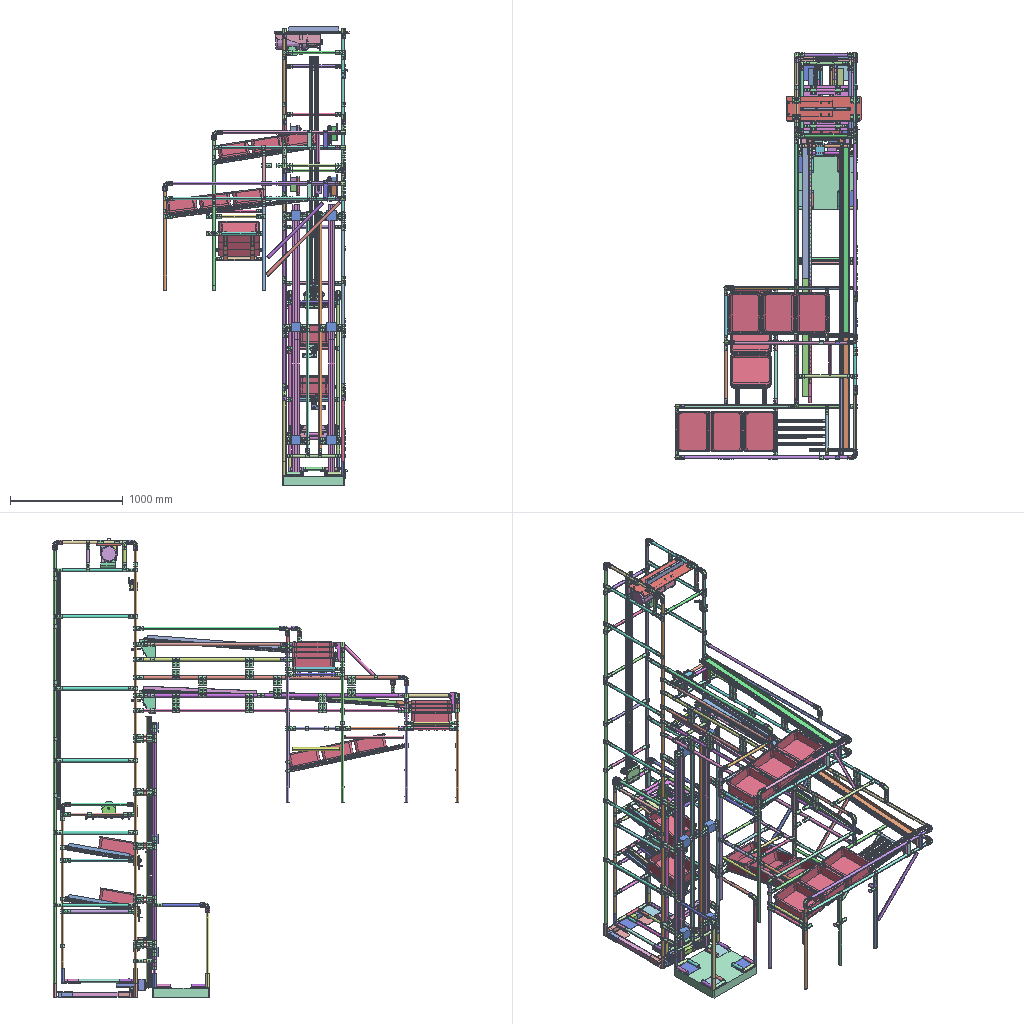Assembly | STEP file | 145 different items | 1167 placed | box 1651 x 3605 x 4075 mm
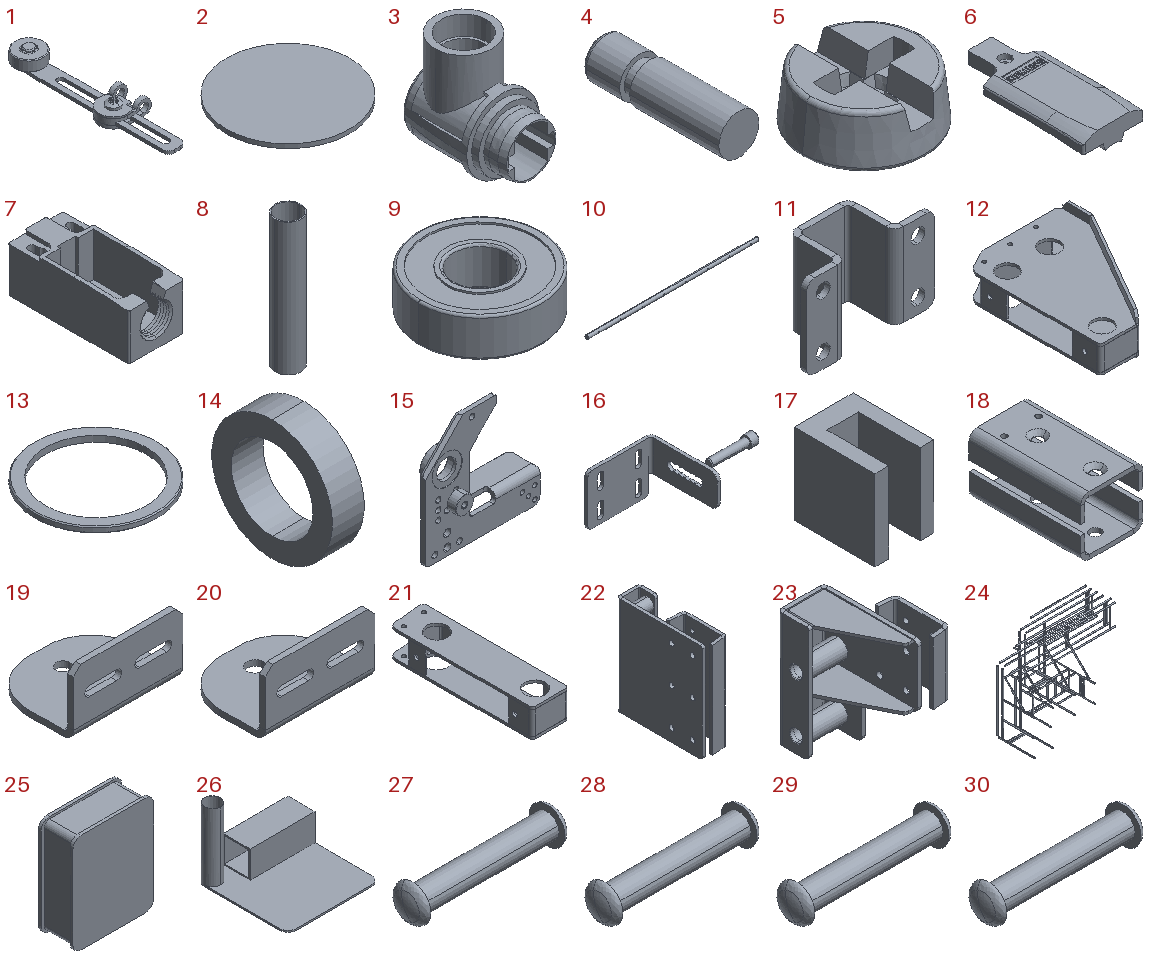Parts list (item | name | quantity | parent item | size | volume):
1 | 2023_07_21_12_39_19_0122 | x2 | in cc_unnamed | 25.5 x 109 x 14 mm | 5452 mm3
2 | 2023_07_21_12_39_19_0126 | x2 | in cc_unnamed | 18 x 18 x 0.6 mm | 152.681 mm3
3 | 2023_07_21_12_39_19_0129 | x2 | in cc_unnamed | 24.025 x 33.5 x 35.012 mm | 7738 mm3
4 | 2023_07_21_12_39_19_0133 | x2 | in cc_unnamed | 7 x 24.6 x 7 mm | 901.225 mm3
5 | 2023_07_21_12_39_19_0137 | x2 | in cc_unnamed | 5.956 x 5.956 x 2.4 mm | 49.622 mm3
6 | 2023_07_21_12_39_19_0141 | x2 | in cc_unnamed | 31 x 68 x 10.875 mm | 10432 mm3
7 | 2023_07_21_12_39_19_0144 | x2 | in cc_unnamed | 31 x 68 x 27 mm | 22352 mm3
8 | 28._28.6X145 | x32 | in SOPORTE DOBLE, Soporte riel_Completo | 28.6 x 28.6 x 145 mm | 14978 mm3
9 | 6202RS | x22 | in POLEA IZAJE ASSY, RODAJA ENSAMBLE, RODAJA ENSAMBLE SUPERIOR, RODAJA FRONTAL | 35 x 35 x 11 mm | 8156 mm3
10 | 6499K55_Shaft for Support Rail_6499K55 | x4 | in RIEL_ASSY | 1200 x 25 x 25 mm | 586134 mm3
11 | ABRAZADERA a | x8 | in ELEVADOR REV 09-03-26 ASSY, ENSAMBLE BASE IZAJE | 77 x 31.7 x 50 mm | 21367 mm3
12 | ACTIVACION MECANICA UPPER RH SLIM V2.1_SLIM V3<Como mecanizada> | x2 | in CAIDA AV3 | 145 x 200 x 60 mm | 208719 mm3
13 | ARANDELA INT. RODAJA | x8 | in RODAJA ENSAMBLE, RODAJA ENSAMBLE SUPERIOR | 18.5 x 18.5 x 0.9 mm | 78.382 mm3
14 | ARANDELA POSTERIOR BALANCIN | x1 | in MECANISMO BALANCIN | 4.76 x 18 x 18 mm | 654.835 mm3
15 | BALANCIN | x1 | in MECANISMO BALANCIN | 130 x 45 x 130 mm | 53768 mm3
16 | BASE ACTIVACION BALANCIN | x1 | in CAIDA AV3 | 205 x 110 x 80 mm | 64247 mm3
17 | BASE GUIA LINEAL_A | x6 | in Soporte riel_Completo | 62 x 85 x 85 mm | 265625 mm3
18 | BASE MICRO | x2 | in cc_unnamed | 38 x 68 x 36 mm | 20484 mm3
19 | BASE POLEA_B_SHEET METAL | x1 | in POLEA IZAJE ASSY | 120 x 100 x 70 mm | 108585 mm3
20 | BASE POLEA_SHEET METAL | x1 | in POLEA IZAJE ASSY | 120 x 100 x 70 mm | 108092 mm3
21 | BASE RIEL SUPERIOR_SLIM V2 | x1 | in CAIDA AV3 | 50 x 199.37 x 39 mm | 75917 mm3
22 | BASE RODILLOS FRONTALES | x1 | in BASE RODILLOS FRONTALES UP | 38.52 x 144.159 x 160 mm | 238623 mm3
23 | BASE RODILLOS SUPERIORES_BASE CONTRA PLACA | x1 | in CANASTA MODIFICACION MECANISMO RETRACTIL | 93.76 x 131.085 x 148 mm | 235886 mm3
24 | CAIDA A V3_Predeterminado<Como mecanizada> | x1 | in CAIDA AV3 | 2864 x 1554 x 1609 mm | 6177747 mm3
25 | CONTENEDOR TORNILLOS | x11 | in CAIDA AV3, CANASTA MODIFICACION MECANISMO RETRACTIL | 292 x 125 x 360 mm | 3821373 mm3
26 | Component1 | x4 | in MB-P | 170 x 170 x 128 mm | 151175 mm3
27 | Component10 | x1 | in Rieles_1 | 25.4 x 6 x 6 mm | 338.091 mm3
28 | Component11 | x1 | in Rieles_1 | 25.4 x 6 x 6 mm | 338.091 mm3
29 | Component12 | x1 | in Rieles_1 | 25.4 x 6 x 6 mm | 338.091 mm3
30 | Component13 | x1 | in Rieles_1 | 25.4 x 6 x 6 mm | 338.091 mm3
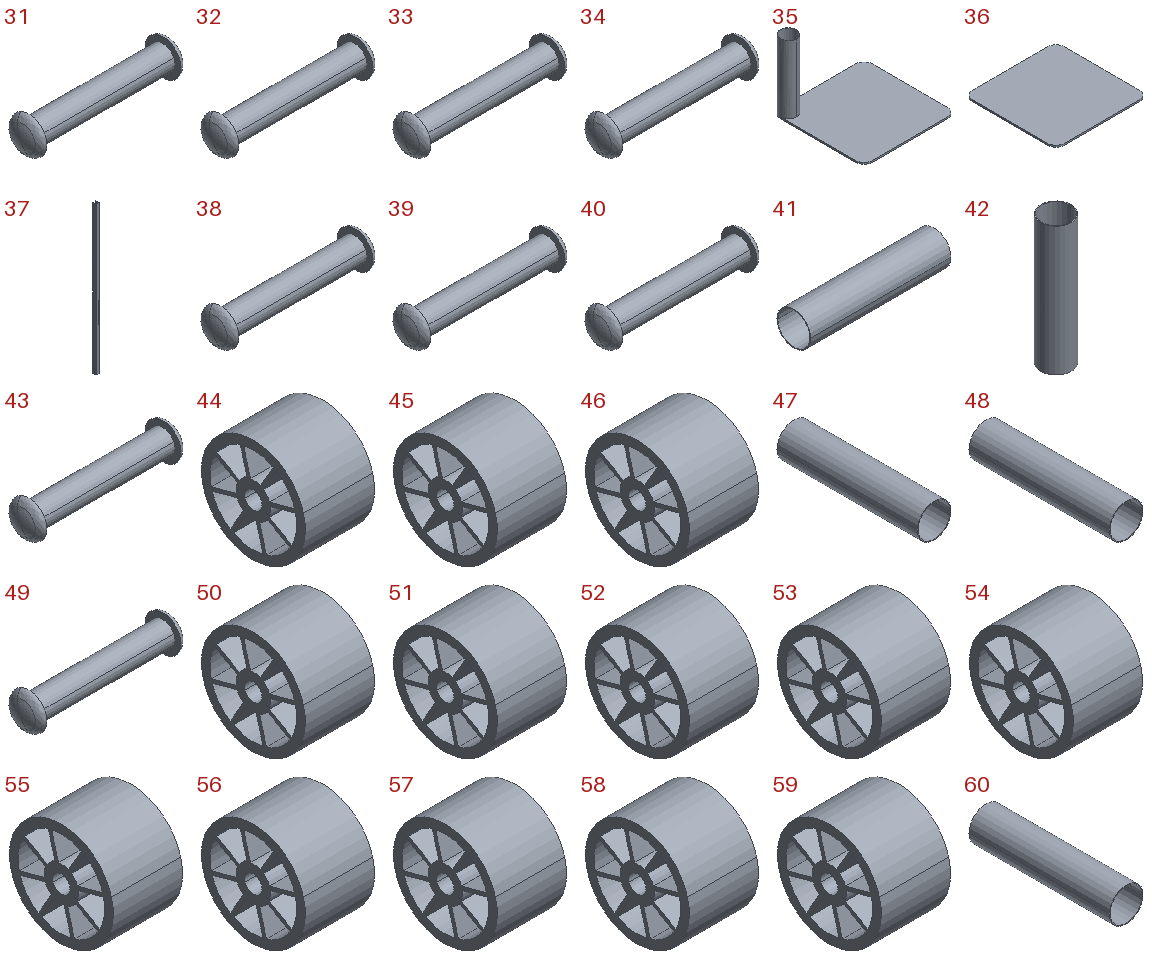31 | Component14 | x1 | in Rieles_1 | 25.4 x 6 x 6 mm | 338.059 mm3
32 | Component15 | x1 | in Rieles_1 | 25.4 x 6 x 6 mm | 338.067 mm3
33 | Component16 | x1 | in Rieles_1 | 25.4 x 6 x 6 mm | 338.067 mm3
34 | Component17 | x1 | in Rieles_1 | 25.4 x 6 x 6 mm | 338.091 mm3
35 | Component1_1 | x4 | in YT-R, YT-R_2 | 170 x 170 x 128 mm | 94175 mm3
36 | Component1_2 | x4 | in YT-L_1, YT-L_3 | 170 x 170 x 3 mm | 86121 mm3
37 | Component2 | x1 | in Rieles_1 | 28.4 x 26.2 x 1238 mm | 123368 mm3
38 | Component25 | x1 | in Rieles_1 | 25.4 x 6 x 6 mm | 338.067 mm3
39 | Component26 | x1 | in Rieles_1 | 25.4 x 6 x 6 mm | 338.067 mm3
40 | Component27 | x1 | in Rieles_1 | 25.4 x 6 x 6 mm | 338.091 mm3
41 | Component2_1 | x4 | in YT-R, YT-R_2 | 125 x 30 x 30 mm | 8054 mm3
42 | Component2_2 | x4 | in YT-L_1, YT-L_3 | 30 x 30 x 125 mm | 8054 mm3
43 | Component3 | x1 | in Rieles_1 | 25.4 x 6 x 6 mm | 338.067 mm3
44 | Component37 | x18 | in Rieles_1 | 20 x 30 x 30 mm | 6699 mm3
45 | Component38 | x1 | in Rieles_1 | 20 x 30 x 30 mm | 6699 mm3
46 | Component39 | x1 | in Rieles_1 | 20 x 30 x 30 mm | 6699 mm3
47 | Component3_1 | x4 | in YT-R, YT-R_2 | 30 x 125 x 30 mm | 8054 mm3
48 | Component3_2 | x4 | in YT-L_1, YT-L_3 | 30 x 125 x 30 mm | 8054 mm3
49 | Component4 | x1 | in Rieles_1 | 25.4 x 6 x 6 mm | 338.067 mm3
50 | Component40 | x1 | in Rieles_1 | 20 x 30 x 30 mm | 6699 mm3
51 | Component41 | x1 | in Rieles_1 | 20 x 30 x 30 mm | 6699 mm3
52 | Component42 | x1 | in Rieles_1 | 20 x 30 x 30 mm | 6699 mm3
53 | Component43 | x1 | in Rieles_1 | 20 x 30 x 30 mm | 6699 mm3
54 | Component44 | x1 | in Rieles_1 | 20 x 30 x 30 mm | 6699 mm3
55 | Component45 | x1 | in Rieles_1 | 20 x 30 x 30 mm | 6699 mm3
56 | Component46 | x1 | in Rieles_1 | 20 x 30 x 30 mm | 6699 mm3
57 | Component47 | x1 | in Rieles_1 | 20 x 30 x 30 mm | 6699 mm3
58 | Component48 | x1 | in Rieles_1 | 20 x 30 x 30 mm | 6699 mm3
59 | Component49 | x1 | in Rieles_1 | 20 x 30 x 30 mm | 6699 mm3
60 | Component4_1 | x4 | in YT-R, YT-R_2 | 30 x 125 x 30 mm | 8054 mm3
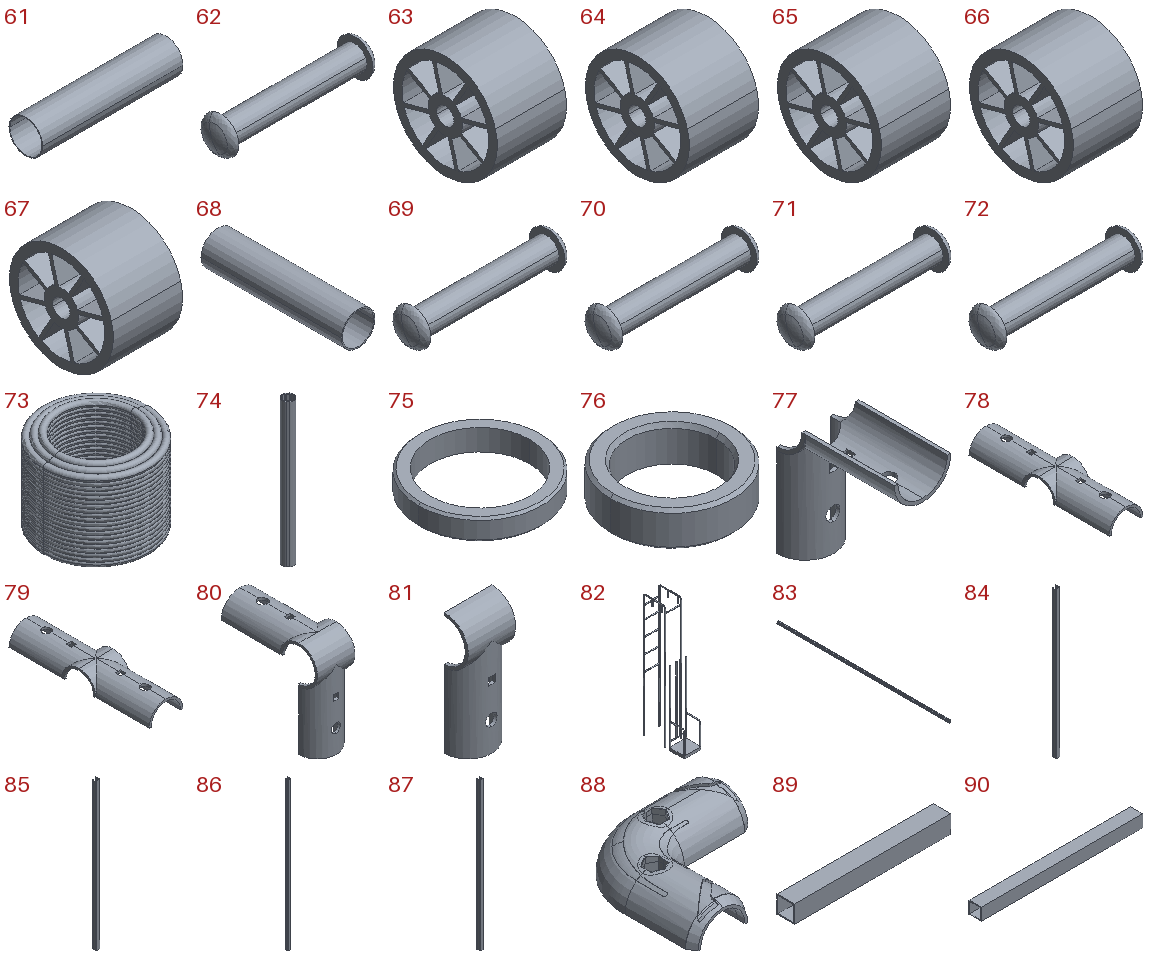61 | Component4_2 | x4 | in YT-L_1, YT-L_3 | 125 x 30 x 30 mm | 8054 mm3
62 | Component5 | x1 | in Rieles_1 | 25.4 x 6 x 6 mm | 338.091 mm3
63 | Component50 | x1 | in Rieles_1 | 20 x 30 x 30 mm | 6699 mm3
64 | Component51 | x1 | in Rieles_1 | 20 x 30 x 30 mm | 6699 mm3
65 | Component52 | x1 | in Rieles_1 | 20 x 30 x 30 mm | 6699 mm3
66 | Component53 | x1 | in Rieles_1 | 20 x 30 x 30 mm | 6699 mm3
67 | Component54 | x117 | in RIEL 1_02, RIEL 2_24, RIEL NIVEL 2-23, RIEL2_02, Rieles_1 | 20 x 30 x 30 mm | 6699 mm3
68 | Component5_1 | x4 | in YT-L_1, YT-L_3 | 30 x 125 x 30 mm | 11388 mm3
69 | Component6 | x1 | in Rieles_1 | 25.4 x 6 x 6 mm | 338.091 mm3
70 | Component7 | x1 | in Rieles_1 | 25.4 x 6 x 6 mm | 338.091 mm3
71 | Component8 | x1 | in Rieles_1 | 25.4 x 6 x 6 mm | 338.091 mm3
72 | Component9 | x1 | in Rieles_1 | 25.4 x 6 x 6 mm | 338.091 mm3
73 | Cable Rep^Pittsburgh Automotive 1300lb remote controlled electric hoist - Representation | x1 | in Pittsburgh Automotive 1300lb remote controlled electric hoist - Representation | 107.694 x 107.694 x 86.428 mm | 372136 mm3
74 | DROP STOP 1 ALUMINUM_Default<As machined> | x2 | in TOPE C1 ALUM | 30 x 30 x 380 mm | 75887 mm3
75 | ESPACIADOR POLEA | x1 | in POLEA IZAJE ASSY | 34.9 x 34.9 x 6 mm | 2006 mm3
76 | ESPACIADOR POLEA 2 | x1 | in POLEA IZAJE ASSY | 21 x 21 x 6 mm | 965.28 mm3
77 | F-A | x22 | in F-A_&_F-C_16, F-A_&_F-C_6 | 32.6 x 67.3 x 67.3 mm | 10224 mm3
78 | F-B | x5 | in F-B_F-B_2 | 32.6 x 134.6 x 16.3 mm | 12017 mm3
79 | F-B_F-B_2-2 | x5 | in F-B_F-B_2 | 32.6 x 134.6 x 16.3 mm | 12017 mm3
80 | F-C | x22 | in F-A_&_F-C_16, F-A_&_F-C_6 | 32.6 x 83.6 x 83.6 mm | 13591 mm3
81 | F-D | x574 | in F-D_F-D_24, F-D_F-D_26, F-D_F-D_27, F-D_F-D_9 | 32.6 x 16.3 x 83.6 mm | 7578 mm3
82 | FRAME ESTRUCTURA REV 3_Predeterminado<Como mecanizada> | x1 | in ELEVADOR REV 09-03-26 ASSY | 552 x 1382 x 4049 mm | 25982334 mm3
83 | FRONT GUIDE_ALUMINUM TUBE ITEM<As machined> | x2 | in GUIAS FRONTALES | 30 x 2110 x 30 mm | 421372 mm3
84 | GALVANIZED RAIL | x1 | in RIEL 1_02 | 28.4 x 26.2 x 999 mm | 99436 mm3
85 | GALVANIZED RAIL 02 | x1 | in RIEL2_02 | 28.4 x 26.2 x 999 mm | 99426 mm3
86 | GALVANIZED RAIL 023 | x1 | in RIEL NIVEL 2-23 | 28.4 x 26.2 x 1678 mm | 167389 mm3
87 | GALVANIZED RAIL 24 | x1 | in RIEL 2_24 | 28.4 x 26.2 x 1218 mm | 121365 mm3
88 | GT-90D | x44 | in HJ13, HJ13_3 | 89.055 x 89.077 x 19.235 mm | 46571 mm3
89 | MB-360X400 | x2 | in ELEVADOR REV 09-03-26 ASSY | 400 x 45 x 45 mm | 170000 mm3
90 | MB-360X600 | x2 | in ELEVADOR REV 09-03-26 ASSY | 600 x 45 x 45 mm | 255000 mm3
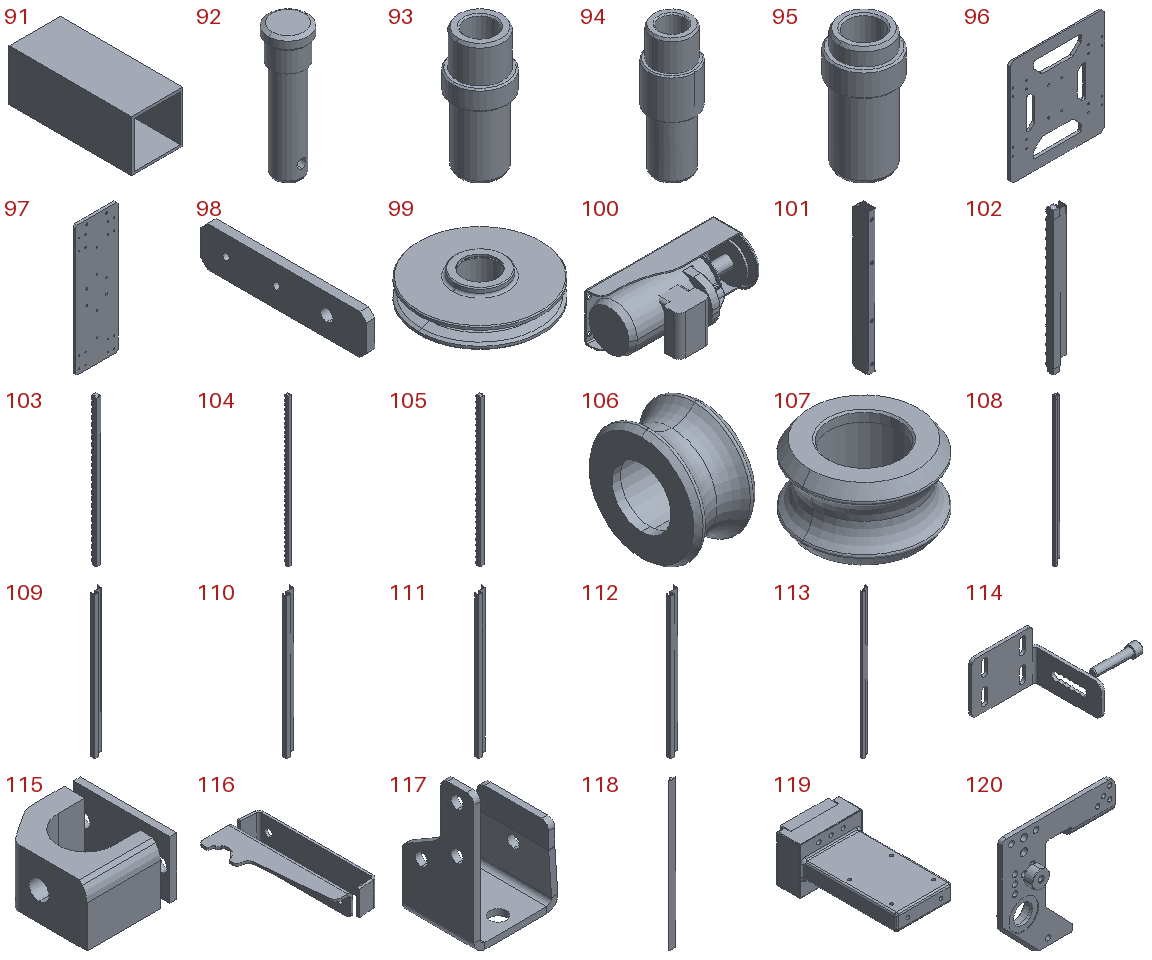91 | MB-P-20 | x4 | in MB-P | 50 x 120 x 50 mm | 57000 mm3
92 | PERNO POLEA_PERNO V2 | x1 | in POLEA IZAJE ASSY | 21 x 21 x 69 mm | 13594 mm3
93 | PERNO RODAJA FRONTAL | x2 | in BASE RODILLOS FRONTALES UP | 19 x 19 x 42.7 mm | 5059 mm3
94 | PERNO RODAJA SUPERIOR | x4 | in RODAJA ENSAMBLE SUPERIOR | 19 x 19 x 52.7 mm | 7077 mm3
95 | PLACA BASE EXCENTRICA | x4 | in RODAJA ENSAMBLE | 18 x 18 x 35.7 mm | 3926 mm3
96 | PLACA BASE IZAJE | x1 | in ENSAMBLE BASE IZAJE | 400 x 12 x 450 mm | 1745930 mm3
97 | PLACA BASE POLIPASTO | x1 | in 97 | 220 x 12 x 665 mm | 1721433 mm3
98 | PLACA SOPORTE GUIA | x2 | in GUIAS FRONTALES | 6.35 x 125 x 30 mm | 22842 mm3
99 | POLEA IZAJE_MAMELON | x1 | in POLEA IZAJE ASSY | 125 x 125 x 35 mm | 205749 mm3
100 | Pittsburgh Hoist^Pittsburgh Automotive 1300lb remote controlled electric hoist - Representation | x1 | in Pittsburgh Automotive 1300lb remote controlled electric hoist - Representation | 415.037 x 200.01 x 149.835 mm | 6132353 mm3
101 | REFUERZO PLACA BASE POLIPASTO | x1 | in 97 | 25.4 x 50.8 x 450 mm | 118043 mm3
102 | RIEL CABINA | x2 | in CANASTA MODIFICACION MECANISMO RETRACTIL | 81.4 x 57.7 x 600 mm | 321427 mm3
103 | RIEL FINAL NLV 1 | x4 | in CAIDA AV3 | 28.4 x 36.2 x 873.5 mm | 257286 mm3
104 | RIEL FINAL NLV 2 | x4 | in CAIDA AV3 | 28.4 x 36.2 x 1308 mm | 381210 mm3
105 | RIEL FINAL NLV 3 | x2 | in CAIDA AV3 | 28.4 x 36.2 x 1045 mm | 307295 mm3
106 | RODAJA D29 | x2 | in RODAJA FRONTAL | 32 x 59.25 x 59.25 mm | 39424 mm3
107 | ROLLER LINEAR GUIDE_01 | x8 | in RODAJA ENSAMBLE, RODAJA ENSAMBLE SUPERIOR | 55.257 x 55.257 x 32 mm | 32346 mm3
108 | Rieles | x1 | in CAIDA AV3 | 81.4 x 57.7 x 1724 mm | 936663 mm3
109 | Rieles_1-21 | x1 | in Rieles_1 | 81.4 x 57.7 x 1164 mm | 303280 mm3
110 | Rieles_1-22 | x1 | in RIEL 1_02 | 81.4 x 57.7 x 1003 mm | 261332 mm3
111 | Rieles_1-24 | x1 | in RIEL 2_24 | 81.4 x 57.7 x 1129 mm | 294161 mm3
112 | Rieles_2-22 | x1 | in RIEL2_02 | 81.4 x 57.7 x 999 mm | 260289 mm3
113 | Rieles_2-23 | x1 | in RIEL NIVEL 2-23 | 81.4 x 57.7 x 1608 mm | 418964 mm3
114 | SIMETRIA BASE ACTIVACION | x1 | in CAIDA AV3 | 205 x 110 x 80 mm | 64247 mm3
115 | SOPORTE BALANCIN | x1 | in MECANISMO BALANCIN | 46.5 x 50 x 30 mm | 35322 mm3
116 | SOPORTE ITEM | x2 | in TOPE C1 ALUM | 83.5 x 174.166 x 35 mm | 61549 mm3
117 | SOPORTE RESORTE 1 | x1 | in CANASTA MODIFICACION MECANISMO RETRACTIL | 35.055 x 30 x 57.6 mm | 7586 mm3
118 | SOPORTE RIEL 25mm | x4 | in RIEL_ASSY | 55 x 21.275 x 1200 mm | 648615 mm3
119 | Sopote_cabina | x2 | in CANASTA MODIFICACION MECANISMO RETRACTIL | 134.1 x 257 x 100 mm | 1531756 mm3
120 | Symmetry BALANCER 01 | x1 | in Symmetry BALANCER MECHANISM | 130 x 45 x 130 mm | 53768 mm3
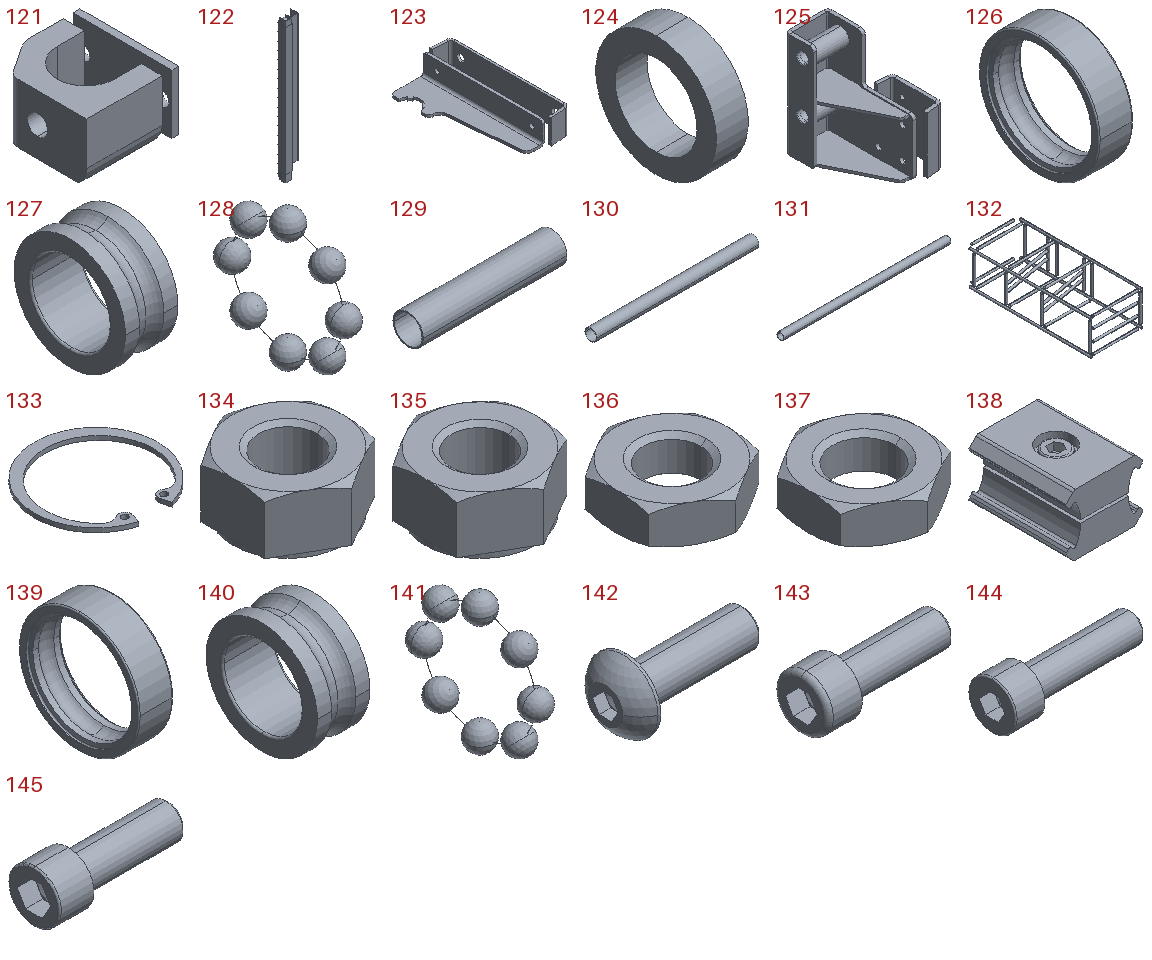121 | Symmetry BALANCER SUPPORT | x1 | in Symmetry BALANCER MECHANISM | 46.5 x 50 x 30 mm | 35322 mm3
122 | Symmetry CABINET RAIL | x2 | in CANASTA MODIFICACION MECANISMO RETRACTIL | 81.4 x 57.7 x 600 mm | 321427 mm3
123 | Symmetry ITEM SUPPORT | x2 | in TOPE C1 ALUM | 83.5 x 174.166 x 35 mm | 61549 mm3
124 | Symmetry REAR WASHER BALANCER | x1 | in Symmetry BALANCER MECHANISM | 4.76 x 18 x 18 mm | 654.835 mm3
125 | Symmetry UPPER ROLLER BASE_COUNTER PLATE BASE | x1 | in CANASTA MODIFICACION MECANISMO RETRACTIL | 93.76 x 131.085 x 148 mm | 235886 mm3
126 | Symmetry skf_bearing_6001_2_01 | x1 | in Symmetry skf_bearing_6001_2 | 8 x 28 x 28 mm | 1280 mm3
127 | Symmetry skf_bearing_6001_2_02 | x1 | in Symmetry skf_bearing_6001_2 | 8 x 17 x 17 mm | 793.588 mm3
128 | Symmetry skf_bearing_6001_2_03 | x1 | in Symmetry skf_bearing_6001_2 | 4.762 x 24.762 x 24.762 mm | 452.339 mm3
129 | TUBO REFUERZO CORTO_Predeterminado<Como mecanizada> | x2 | in REFUERZO CORTO | 135.6 x 28.6 x 28.6 mm | 14007 mm3
130 | TUBO REFUERZO LONGITUDINAL.2_Predeterminado<Como mecanizada> | x6 | in REFUERZO FRONTAL CABINA | 395 x 28.6 x 28.6 mm | 40802 mm3
131 | TUBO REFUERZO LONGITUDINAL_Predeterminado<Como mecanizada> | x12 | in REFUERZO LONGITUDINAL | 685 x 28.6 x 28.6 mm | 70757 mm3
132 | TUBOS CANASTA_Predeterminado<Como mecanizada> | x1 | in CANASTA MODIFICACION MECANISMO RETRACTIL | 675 x 1600 x 455 mm | 1954173 mm3
133 | basic internal retaining ring_wti.25698_Truarc N5000-137 - S1.375 | x4 | in POLEA IZAJE ASSY, RODAJA FRONTAL | 37.109 x 36.419 x 1.27 mm | 328.567 mm3
134 | hex nut style 1 gradeab_iso_ISO - 4032 - M10 - W - N | x4 | in ENSAMBLE BASE IZAJE | 16 x 18.475 x 8.4 mm | 1357 mm3
135 | hex nut style 1 gradeab_iso_ISO - 4032 - M8 - W - N | x16 | in ENSAMBLE BASE IZAJE | 13 x 15.011 x 6.8 mm | 731.665 mm3
136 | hex thin nut chamfered gradeab_iso.246_ISO - 4035 - M5 - N | x1 | in MECANISMO BALANCIN | 8 x 9.238 x 2.7 mm | 109.405 mm3
137 | hex thin nut chamfered gradeab_iso_ISO - 4035 - M12 - N | x2 | in CAIDA AV3 | 18 x 20.785 x 6 mm | 1161 mm3
138 | - | x6 | in GUIAS FRONTALES | 30.2 x 38 x 24 mm | 19567 mm3
139 | skf_bearing_6001_2_01 | x1 | in skf_bearing_6001_2 | 8 x 28 x 28 mm | 1280 mm3
140 | skf_bearing_6001_2_02 | x1 | in skf_bearing_6001_2 | 8 x 17 x 17 mm | 793.588 mm3
141 | skf_bearing_6001_2_03 | x1 | in skf_bearing_6001_2 | 4.762 x 24.762 x 24.762 mm | 452.339 mm3
142 | socket button head screw_iso_ISO 7380 - M5 x 16 - 16N | x1 | in MECANISMO BALANCIN | 18.75 x 9.5 x 9.5 mm | 437.534 mm3
143 | socket head cap screw_iso.3336_ISO 4762 M10 x 30 - 30N | x4 | in ENSAMBLE BASE IZAJE | 40 x 16 x 16 mm | 4009 mm3
144 | socket head cap screw_iso.3336_ISO 4762 M8 x 30 - 30N | x16 | in ENSAMBLE BASE IZAJE | 38 x 13 x 13 mm | 2418 mm3
145 | socket head cap screw_iso_ISO 4762 M12 x 35 - 35N | x1 | in CANASTA MODIFICACION MECANISMO RETRACTIL | 47 x 18 x 18 mm | 6384 mm3